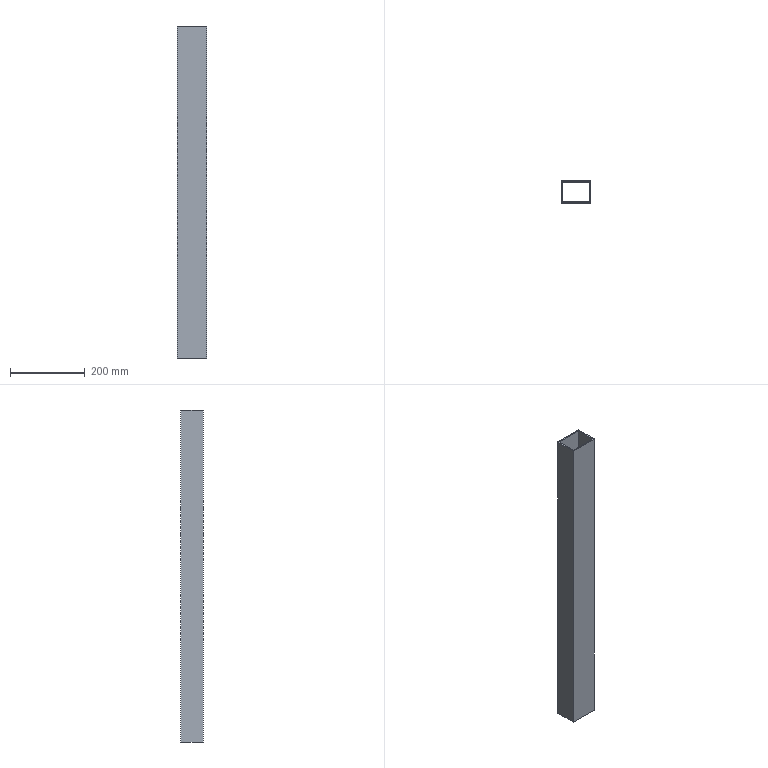Part | STEP file | Guide wheel mechanism revised.sldasm-Part-8 | 1 solid | 10 faces | box 80 x 60 x 890 mm | volume 715560 mm3 | plane 10
STEP:
#1=CARTESIAN_POINT('',(-405.,1970.,445.));
#2=VERTEX_POINT('',#1);
#3=CARTESIAN_POINT('',(-485.,1970.,445.));
#4=VERTEX_POINT('',#3);
#5=CARTESIAN_POINT('',(-485.,1970.,445.));
#6=DIRECTION('',(-1.,0.,0.));
#7=VECTOR('',#6,1000.);
#8=LINE('',#5,#7);
#9=EDGE_CURVE('',#2,#4,#8,.T.);
#10=ORIENTED_EDGE('',*,*,#9,.F.);
#11=CARTESIAN_POINT('',(-405.,1970.,-445.));
#12=VERTEX_POINT('',#11);
#13=CARTESIAN_POINT('',(-405.,1970.,545.));
#14=DIRECTION('',(0.,0.,-1.));
#15=VECTOR('',#14,1000.);
#16=LINE('',#13,#15);
#17=EDGE_CURVE('',#2,#12,#16,.T.);
#18=ORIENTED_EDGE('',*,*,#17,.T.);
#19=CARTESIAN_POINT('',(-485.,1970.,-445.));
#20=VERTEX_POINT('',#19);
#21=CARTESIAN_POINT('',(-485.,1970.,-445.));
#22=DIRECTION('',(-1.,0.,0.));
#23=VECTOR('',#22,1000.);
#24=LINE('',#21,#23);
#25=EDGE_CURVE('',#12,#20,#24,.T.);
#26=ORIENTED_EDGE('',*,*,#25,.T.);
#27=CARTESIAN_POINT('',(-485.,1970.,545.));
#28=DIRECTION('',(0.,0.,-1.));
#29=VECTOR('',#28,1000.);
#30=LINE('',#27,#29);
#31=EDGE_CURVE('',#4,#20,#30,.T.);
#32=ORIENTED_EDGE('',*,*,#31,.F.);
#33=EDGE_LOOP('',(#10,#18,#26,#32));
#34=FACE_OUTER_BOUND('',#33,.T.);
#35=CARTESIAN_POINT('',(-485.,1970.,545.));
#36=DIRECTION('',(0.,-1.,0.));
#37=DIRECTION('',(0.,0.,-1.));
#38=AXIS2_PLACEMENT_3D('',#35,#36,#37);
#39=PLANE('',#38);
#40=ADVANCED_FACE('',(#34),#39,.F.);
#41=CARTESIAN_POINT('',(-405.,1910.,445.));
#42=VERTEX_POINT('',#41);
#43=CARTESIAN_POINT('',(-405.,1970.,445.));
#44=DIRECTION('',(0.,1.,0.));
#45=VECTOR('',#44,1000.);
#46=LINE('',#43,#45);
#47=EDGE_CURVE('',#42,#2,#46,.T.);
#48=ORIENTED_EDGE('',*,*,#47,.F.);
#49=CARTESIAN_POINT('',(-405.,1910.,-445.));
#50=VERTEX_POINT('',#49);
#51=CARTESIAN_POINT('',(-405.,1910.,545.));
#52=DIRECTION('',(0.,0.,-1.));
#53=VECTOR('',#52,1000.);
#54=LINE('',#51,#53);
#55=EDGE_CURVE('',#42,#50,#54,.T.);
#56=ORIENTED_EDGE('',*,*,#55,.T.);
#57=CARTESIAN_POINT('',(-405.,1970.,-445.));
#58=DIRECTION('',(0.,1.,0.));
#59=VECTOR('',#58,1000.);
#60=LINE('',#57,#59);
#61=EDGE_CURVE('',#50,#12,#60,.T.);
#62=ORIENTED_EDGE('',*,*,#61,.T.);
#63=ORIENTED_EDGE('',*,*,#17,.F.);
#64=EDGE_LOOP('',(#48,#56,#62,#63));
#65=FACE_OUTER_BOUND('',#64,.T.);
#66=CARTESIAN_POINT('',(-405.,1970.,545.));
#67=DIRECTION('',(-1.,0.,0.));
#68=DIRECTION('',(0.,0.,1.));
#69=AXIS2_PLACEMENT_3D('',#66,#67,#68);
#70=PLANE('',#69);
#71=ADVANCED_FACE('',(#65),#70,.F.);
#72=CARTESIAN_POINT('',(-485.,1910.,445.));
#73=VERTEX_POINT('',#72);
#74=CARTESIAN_POINT('',(-485.,1910.,445.));
#75=DIRECTION('',(1.,0.,0.));
#76=VECTOR('',#75,1000.);
#77=LINE('',#74,#76);
#78=EDGE_CURVE('',#73,#42,#77,.T.);
#79=ORIENTED_EDGE('',*,*,#78,.F.);
#80=CARTESIAN_POINT('',(-485.,1910.,-445.));
#81=VERTEX_POINT('',#80);
#82=CARTESIAN_POINT('',(-485.,1910.,545.));
#83=DIRECTION('',(0.,0.,-1.));
#84=VECTOR('',#83,1000.);
#85=LINE('',#82,#84);
#86=EDGE_CURVE('',#73,#81,#85,.T.);
#87=ORIENTED_EDGE('',*,*,#86,.T.);
#88=CARTESIAN_POINT('',(-485.,1910.,-445.));
#89=DIRECTION('',(1.,0.,0.));
#90=VECTOR('',#89,1000.);
#91=LINE('',#88,#90);
#92=EDGE_CURVE('',#81,#50,#91,.T.);
#93=ORIENTED_EDGE('',*,*,#92,.T.);
#94=ORIENTED_EDGE('',*,*,#55,.F.);
#95=EDGE_LOOP('',(#79,#87,#93,#94));
#96=FACE_OUTER_BOUND('',#95,.T.);
#97=CARTESIAN_POINT('',(-485.,1910.,545.));
#98=DIRECTION('',(0.,1.,0.));
#99=DIRECTION('',(0.,0.,1.));
#100=AXIS2_PLACEMENT_3D('',#97,#98,#99);
#101=PLANE('',#100);
#102=ADVANCED_FACE('',(#96),#101,.F.);
#103=CARTESIAN_POINT('',(-485.,1970.,445.));
#104=DIRECTION('',(0.,-1.,0.));
#105=VECTOR('',#104,1000.);
#106=LINE('',#103,#105);
#107=EDGE_CURVE('',#4,#73,#106,.T.);
#108=ORIENTED_EDGE('',*,*,#107,.F.);
#109=ORIENTED_EDGE('',*,*,#31,.T.);
#110=CARTESIAN_POINT('',(-485.,1970.,-445.));
#111=DIRECTION('',(0.,-1.,0.));
#112=VECTOR('',#111,1000.);
#113=LINE('',#110,#112);
#114=EDGE_CURVE('',#20,#81,#113,.T.);
#115=ORIENTED_EDGE('',*,*,#114,.T.);
#116=ORIENTED_EDGE('',*,*,#86,.F.);
#117=EDGE_LOOP('',(#108,#109,#115,#116));
#118=FACE_OUTER_BOUND('',#117,.T.);
#119=CARTESIAN_POINT('',(-485.,1970.,545.));
#120=DIRECTION('',(1.,0.,0.));
#121=DIRECTION('',(0.,0.,-1.));
#122=AXIS2_PLACEMENT_3D('',#119,#120,#121);
#123=PLANE('',#122);
#124=ADVANCED_FACE('',(#118),#123,.F.);
#125=ORIENTED_EDGE('',*,*,#114,.F.);
#126=ORIENTED_EDGE('',*,*,#25,.F.);
#127=ORIENTED_EDGE('',*,*,#61,.F.);
#128=ORIENTED_EDGE('',*,*,#92,.F.);
#129=EDGE_LOOP('',(#125,#126,#127,#128));
#130=FACE_OUTER_BOUND('',#129,.T.);
#131=CARTESIAN_POINT('',(-482.,1967.,-445.));
#132=VERTEX_POINT('',#131);
#133=CARTESIAN_POINT('',(-482.,1913.,-445.));
#134=VERTEX_POINT('',#133);
#135=CARTESIAN_POINT('',(-482.,1967.,-445.));
#136=DIRECTION('',(0.,-1.,0.));
#137=VECTOR('',#136,1000.);
#138=LINE('',#135,#137);
#139=EDGE_CURVE('',#132,#134,#138,.T.);
#140=ORIENTED_EDGE('',*,*,#139,.T.);
#141=CARTESIAN_POINT('',(-408.,1913.,-445.));
#142=VERTEX_POINT('',#141);
#143=CARTESIAN_POINT('',(-482.,1913.,-445.));
#144=DIRECTION('',(1.,0.,0.));
#145=VECTOR('',#144,1000.);
#146=LINE('',#143,#145);
#147=EDGE_CURVE('',#134,#142,#146,.T.);
#148=ORIENTED_EDGE('',*,*,#147,.T.);
#149=CARTESIAN_POINT('',(-408.,1967.,-445.));
#150=VERTEX_POINT('',#149);
#151=CARTESIAN_POINT('',(-408.,1967.,-445.));
#152=DIRECTION('',(0.,1.,0.));
#153=VECTOR('',#152,1000.);
#154=LINE('',#151,#153);
#155=EDGE_CURVE('',#142,#150,#154,.T.);
#156=ORIENTED_EDGE('',*,*,#155,.T.);
#157=CARTESIAN_POINT('',(-482.,1967.,-445.));
#158=DIRECTION('',(-1.,0.,0.));
#159=VECTOR('',#158,1000.);
#160=LINE('',#157,#159);
#161=EDGE_CURVE('',#150,#132,#160,.T.);
#162=ORIENTED_EDGE('',*,*,#161,.T.);
#163=EDGE_LOOP('',(#140,#148,#156,#162));
#164=FACE_BOUND('',#163,.T.);
#165=CARTESIAN_POINT('',(0.,0.,-445.));
#166=DIRECTION('',(0.,0.,1.));
#167=DIRECTION('',(1.,0.,0.));
#168=AXIS2_PLACEMENT_3D('',#165,#166,#167);
#169=PLANE('',#168);
#170=ADVANCED_FACE('',(#130,#164),#169,.F.);
#171=CARTESIAN_POINT('',(-408.,1967.,445.));
#172=VERTEX_POINT('',#171);
#173=CARTESIAN_POINT('',(-408.,1967.,545.));
#174=DIRECTION('',(0.,0.,-1.));
#175=VECTOR('',#174,1000.);
#176=LINE('',#173,#175);
#177=EDGE_CURVE('',#172,#150,#176,.T.);
#178=ORIENTED_EDGE('',*,*,#177,.F.);
#179=CARTESIAN_POINT('',(-482.,1967.,445.));
#180=VERTEX_POINT('',#179);
#181=CARTESIAN_POINT('',(-482.,1967.,445.));
#182=DIRECTION('',(-1.,0.,0.));
#183=VECTOR('',#182,1000.);
#184=LINE('',#181,#183);
#185=EDGE_CURVE('',#172,#180,#184,.T.);
#186=ORIENTED_EDGE('',*,*,#185,.T.);
#187=CARTESIAN_POINT('',(-482.,1967.,545.));
#188=DIRECTION('',(0.,0.,-1.));
#189=VECTOR('',#188,1000.);
#190=LINE('',#187,#189);
#191=EDGE_CURVE('',#180,#132,#190,.T.);
#192=ORIENTED_EDGE('',*,*,#191,.T.);
#193=ORIENTED_EDGE('',*,*,#161,.F.);
#194=EDGE_LOOP('',(#178,#186,#192,#193));
#195=FACE_OUTER_BOUND('',#194,.T.);
#196=CARTESIAN_POINT('',(-482.,1967.,545.));
#197=DIRECTION('',(0.,-1.,0.));
#198=DIRECTION('',(0.,0.,-1.));
#199=AXIS2_PLACEMENT_3D('',#196,#197,#198);
#200=PLANE('',#199);
#201=ADVANCED_FACE('',(#195),#200,.T.);
#202=CARTESIAN_POINT('',(-408.,1913.,445.));
#203=VERTEX_POINT('',#202);
#204=CARTESIAN_POINT('',(-408.,1913.,545.));
#205=DIRECTION('',(0.,0.,-1.));
#206=VECTOR('',#205,1000.);
#207=LINE('',#204,#206);
#208=EDGE_CURVE('',#203,#142,#207,.T.);
#209=ORIENTED_EDGE('',*,*,#208,.F.);
#210=CARTESIAN_POINT('',(-408.,1967.,445.));
#211=DIRECTION('',(0.,1.,0.));
#212=VECTOR('',#211,1000.);
#213=LINE('',#210,#212);
#214=EDGE_CURVE('',#203,#172,#213,.T.);
#215=ORIENTED_EDGE('',*,*,#214,.T.);
#216=ORIENTED_EDGE('',*,*,#177,.T.);
#217=ORIENTED_EDGE('',*,*,#155,.F.);
#218=EDGE_LOOP('',(#209,#215,#216,#217));
#219=FACE_OUTER_BOUND('',#218,.T.);
#220=CARTESIAN_POINT('',(-408.,1967.,545.));
#221=DIRECTION('',(-1.,0.,0.));
#222=DIRECTION('',(0.,-1.,0.));
#223=AXIS2_PLACEMENT_3D('',#220,#221,#222);
#224=PLANE('',#223);
#225=ADVANCED_FACE('',(#219),#224,.T.);
#226=CARTESIAN_POINT('',(-482.,1913.,445.));
#227=VERTEX_POINT('',#226);
#228=CARTESIAN_POINT('',(-482.,1913.,545.));
#229=DIRECTION('',(0.,0.,-1.));
#230=VECTOR('',#229,1000.);
#231=LINE('',#228,#230);
#232=EDGE_CURVE('',#227,#134,#231,.T.);
#233=ORIENTED_EDGE('',*,*,#232,.F.);
#234=CARTESIAN_POINT('',(-482.,1913.,445.));
#235=DIRECTION('',(1.,0.,0.));
#236=VECTOR('',#235,1000.);
#237=LINE('',#234,#236);
#238=EDGE_CURVE('',#227,#203,#237,.T.);
#239=ORIENTED_EDGE('',*,*,#238,.T.);
#240=ORIENTED_EDGE('',*,*,#208,.T.);
#241=ORIENTED_EDGE('',*,*,#147,.F.);
#242=EDGE_LOOP('',(#233,#239,#240,#241));
#243=FACE_OUTER_BOUND('',#242,.T.);
#244=CARTESIAN_POINT('',(-482.,1913.,545.));
#245=DIRECTION('',(0.,1.,0.));
#246=DIRECTION('',(0.,0.,1.));
#247=AXIS2_PLACEMENT_3D('',#244,#245,#246);
#248=PLANE('',#247);
#249=ADVANCED_FACE('',(#243),#248,.T.);
#250=ORIENTED_EDGE('',*,*,#191,.F.);
#251=CARTESIAN_POINT('',(-482.,1967.,445.));
#252=DIRECTION('',(0.,-1.,0.));
#253=VECTOR('',#252,1000.);
#254=LINE('',#251,#253);
#255=EDGE_CURVE('',#180,#227,#254,.T.);
#256=ORIENTED_EDGE('',*,*,#255,.T.);
#257=ORIENTED_EDGE('',*,*,#232,.T.);
#258=ORIENTED_EDGE('',*,*,#139,.F.);
#259=EDGE_LOOP('',(#250,#256,#257,#258));
#260=FACE_OUTER_BOUND('',#259,.T.);
#261=CARTESIAN_POINT('',(-482.,1967.,545.));
#262=DIRECTION('',(1.,0.,0.));
#263=DIRECTION('',(0.,1.,0.));
#264=AXIS2_PLACEMENT_3D('',#261,#262,#263);
#265=PLANE('',#264);
#266=ADVANCED_FACE('',(#260),#265,.T.);
#267=ORIENTED_EDGE('',*,*,#255,.F.);
#268=ORIENTED_EDGE('',*,*,#185,.F.);
#269=ORIENTED_EDGE('',*,*,#214,.F.);
#270=ORIENTED_EDGE('',*,*,#238,.F.);
#271=EDGE_LOOP('',(#267,#268,#269,#270));
#272=FACE_BOUND('',#271,.T.);
#273=ORIENTED_EDGE('',*,*,#9,.T.);
#274=ORIENTED_EDGE('',*,*,#107,.T.);
#275=ORIENTED_EDGE('',*,*,#78,.T.);
#276=ORIENTED_EDGE('',*,*,#47,.T.);
#277=EDGE_LOOP('',(#273,#274,#275,#276));
#278=FACE_OUTER_BOUND('',#277,.T.);
#279=CARTESIAN_POINT('',(-405.,1970.,445.));
#280=DIRECTION('',(0.,0.,1.));
#281=DIRECTION('',(1.,0.,0.));
#282=AXIS2_PLACEMENT_3D('',#279,#280,#281);
#283=PLANE('',#282);
#284=ADVANCED_FACE('',(#272,#278),#283,.T.);
#285=CLOSED_SHELL('',(#40,#71,#102,#124,#170,#201,#225,#249,#266,#284));
#286=MANIFOLD_SOLID_BREP('',#285);
#287=CARTESIAN_POINT('',(0.,0.,0.));
#288=DIRECTION('',(0.,0.,1.));
#289=DIRECTION('',(1.,0.,0.));
#290=AXIS2_PLACEMENT_3D('',#287,#288,#289);
#291=(LENGTH_UNIT()NAMED_UNIT(*)SI_UNIT(.MILLI.,.METRE.));
#292=UNCERTAINTY_MEASURE_WITH_UNIT(LENGTH_MEASURE(0.00001),#291,'','');
#293=(NAMED_UNIT(*)PLANE_ANGLE_UNIT()SI_UNIT($,.RADIAN.));
#294=(NAMED_UNIT(*)SI_UNIT($,.STERADIAN.)SOLID_ANGLE_UNIT());
#295=(GEOMETRIC_REPRESENTATION_CONTEXT(3)GLOBAL_UNCERTAINTY_ASSIGNED_CONTEXT((#292))GLOBAL_UNIT_ASSIGNED_CONTEXT((#291,#293,#294))REPRESENTATION_CONTEXT('',''));
#296=ADVANCED_BREP_SHAPE_REPRESENTATION('',(#286,#290),#295);